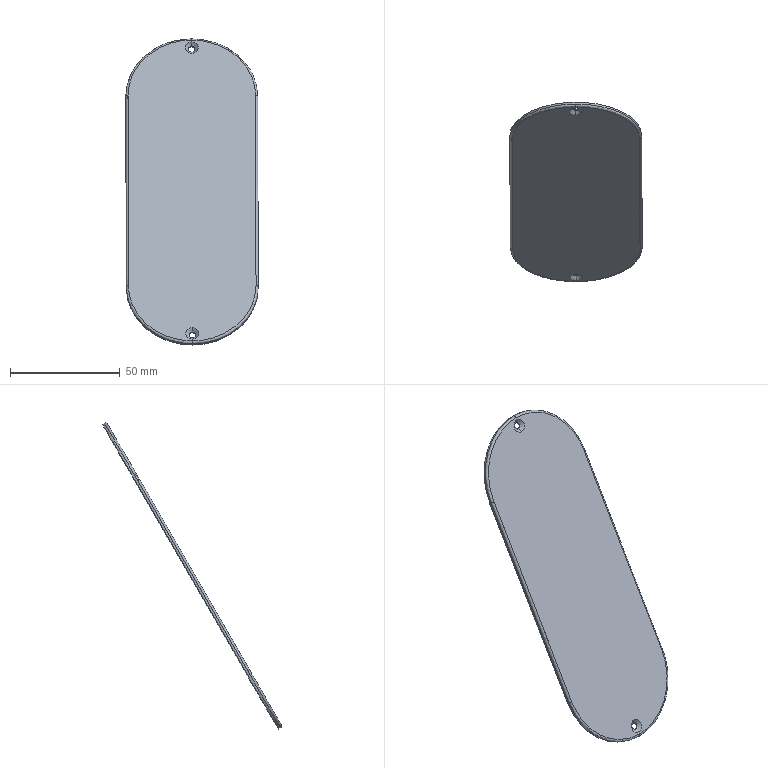Part | SolidWorks | features BaseBody 1 | 1 solid | 22 faces | box 60.221 x 81.366 x 139.198 mm | volume 17515 mm3 | cylinder 10 | spline 4 | cone 4 | plane 4 | commonest cylinder face diameters 3 x4 2 x3 60 x3
STEP:
#1=CARTESIAN_POINT('',(743.209,-1.322,-30.446));
#2=VERTEX_POINT('',#1);
#3=CARTESIAN_POINT('',(743.144,-1.322,-30.446));
#4=VERTEX_POINT('',#3);
#5=CARTESIAN_POINT('',(743.144,13.678,-4.465));
#6=DIRECTION('',(-0.003769,0.866,-0.5));
#7=DIRECTION('',(0.,-0.5,-0.866));
#8=AXIS2_PLACEMENT_3D('',#5,#6,#7);
#9=CIRCLE('',#8,30.);
#10=EDGE_CURVE('',#2,#4,#9,.T.);
#11=ORIENTED_EDGE('',*,*,#10,.F.);
#12=CARTESIAN_POINT('',(743.211,-1.688,-29.08));
#13=VERTEX_POINT('',#12);
#14=CARTESIAN_POINT('',(743.207,-0.8215,-29.58));
#15=DIRECTION('',(-1.,-0.004352,0.000000001));
#16=DIRECTION('',(0.002176,-0.5,-0.866));
#17=AXIS2_PLACEMENT_3D('',#14,#15,#16);
#18=CIRCLE('',#17,1.);
#19=EDGE_CURVE('',#2,#13,#18,.T.);
#20=ORIENTED_EDGE('',*,*,#19,.T.);
#21=CARTESIAN_POINT('',(714.148,12.686,-3.965));
#22=VERTEX_POINT('',#21);
#23=CARTESIAN_POINT('',(743.211,-1.688,-29.08));
#24=CARTESIAN_POINT('',(726.223,-1.761,-29.08));
#25=CARTESIAN_POINT('',(714.185,4.192,-18.677));
#26=CARTESIAN_POINT('',(714.148,12.686,-3.965));
#27=(BOUNDED_CURVE()B_SPLINE_CURVE(3,(#23,#24,#25,#26),.UNSPECIFIED.,.F.,.F.)B_SPLINE_CURVE_WITH_KNOTS((4,4),(0.,1.),.UNSPECIFIED.)CURVE()GEOMETRIC_REPRESENTATION_ITEM()RATIONAL_B_SPLINE_CURVE((1.,0.8047,0.8047,1.))REPRESENTATION_ITEM(''));
#28=EDGE_CURVE('',#13,#22,#27,.T.);
#29=ORIENTED_EDGE('',*,*,#28,.T.);
#30=CARTESIAN_POINT('',(714.144,12.686,-3.965));
#31=VERTEX_POINT('',#30);
#32=CARTESIAN_POINT('',(714.144,13.552,-4.465));
#33=DIRECTION('',(0.002176,-0.5,-0.866));
#34=DIRECTION('',(-1.,-0.004352,0.000000001));
#35=AXIS2_PLACEMENT_3D('',#32,#33,#34);
#36=CIRCLE('',#35,1.);
#37=EDGE_CURVE('',#22,#31,#36,.T.);
#38=ORIENTED_EDGE('',*,*,#37,.T.);
#39=CARTESIAN_POINT('',(713.144,13.548,-4.465));
#40=VERTEX_POINT('',#39);
#41=CARTESIAN_POINT('',(714.144,13.552,-4.465));
#42=DIRECTION('',(0.002176,-0.5,-0.866));
#43=DIRECTION('',(-1.,-0.004352,0.000000001));
#44=AXIS2_PLACEMENT_3D('',#41,#42,#43);
#45=CIRCLE('',#44,1.);
#46=EDGE_CURVE('',#31,#40,#45,.T.);
#47=ORIENTED_EDGE('',*,*,#46,.T.);
#48=CARTESIAN_POINT('',(743.144,13.678,-4.465));
#49=DIRECTION('',(-0.003769,0.866,-0.5));
#50=DIRECTION('',(0.,-0.5,-0.866));
#51=AXIS2_PLACEMENT_3D('',#48,#49,#50);
#52=CIRCLE('',#51,30.);
#53=EDGE_CURVE('',#4,#40,#52,.T.);
#54=ORIENTED_EDGE('',*,*,#53,.F.);
#55=EDGE_LOOP('',(#11,#20,#29,#38,#47,#54));
#56=FACE_OUTER_BOUND('',#55,.T.);
#57=CARTESIAN_POINT('',(743.209,-1.322,-30.446));
#58=CARTESIAN_POINT('',(725.636,-1.398,-30.446));
#59=CARTESIAN_POINT('',(713.182,4.761,-19.684));
#60=CARTESIAN_POINT('',(713.144,13.548,-4.465));
#61=CARTESIAN_POINT('',(743.211,-1.829,-30.153));
#62=CARTESIAN_POINT('',(725.638,-1.905,-30.153));
#63=CARTESIAN_POINT('',(713.185,4.254,-19.391));
#64=CARTESIAN_POINT('',(713.146,13.04,-4.172));
#65=CARTESIAN_POINT('',(743.212,-1.98,-29.587));
#66=CARTESIAN_POINT('',(725.881,-2.056,-29.587));
#67=CARTESIAN_POINT('',(713.6,4.018,-18.974));
#68=CARTESIAN_POINT('',(713.562,12.684,-3.965));
#69=CARTESIAN_POINT('',(743.211,-1.688,-29.08));
#70=CARTESIAN_POINT('',(726.223,-1.761,-29.08));
#71=CARTESIAN_POINT('',(714.185,4.192,-18.677));
#72=CARTESIAN_POINT('',(714.148,12.686,-3.965));
#73=(BOUNDED_SURFACE()B_SPLINE_SURFACE(3,3,((#57,#58,#59,#60),(#61,#62,#63,#64),(#65,#66,#67,#68),(#69,#70,#71,#72)),.UNSPECIFIED.,.F.,.F.,.T.)B_SPLINE_SURFACE_WITH_KNOTS((4,4),(4,4),(0.,1.),(0.,1.),.UNSPECIFIED.)GEOMETRIC_REPRESENTATION_ITEM()RATIONAL_B_SPLINE_SURFACE(((1.,0.8047,0.8047,1.),(0.8047,0.6476,0.6476,0.8047),(0.8047,0.6476,0.6476,0.8047),(1.,0.8047,0.8047,1.)))REPRESENTATION_ITEM('')SURFACE());
#74=ADVANCED_FACE('',(#56),#73,.T.);
#75=CARTESIAN_POINT('',(742.861,78.678,108.118));
#76=VERTEX_POINT('',#75);
#77=CARTESIAN_POINT('',(772.926,63.808,82.137));
#78=VERTEX_POINT('',#77);
#79=CARTESIAN_POINT('',(742.926,63.678,82.137));
#80=DIRECTION('',(-0.003769,0.866,-0.5));
#81=DIRECTION('',(0.,-0.5,-0.866));
#82=AXIS2_PLACEMENT_3D('',#79,#80,#81);
#83=CIRCLE('',#82,30.);
#84=EDGE_CURVE('',#76,#78,#83,.T.);
#85=ORIENTED_EDGE('',*,*,#84,.F.);
#86=CARTESIAN_POINT('',(742.867,77.312,107.752));
#87=VERTEX_POINT('',#86);
#88=CARTESIAN_POINT('',(742.863,78.178,107.252));
#89=DIRECTION('',(1.,0.004352,-0.000000001));
#90=DIRECTION('',(-0.002176,0.5,0.866));
#91=AXIS2_PLACEMENT_3D('',#88,#89,#90);
#92=CIRCLE('',#91,1.);
#93=EDGE_CURVE('',#76,#87,#92,.T.);
#94=ORIENTED_EDGE('',*,*,#93,.T.);
#95=CARTESIAN_POINT('',(771.93,62.938,82.637));
#96=VERTEX_POINT('',#95);
#97=CARTESIAN_POINT('',(742.867,77.312,107.752));
#98=CARTESIAN_POINT('',(759.855,77.386,107.752));
#99=CARTESIAN_POINT('',(771.893,71.432,97.349));
#100=CARTESIAN_POINT('',(771.93,62.938,82.637));
#101=(BOUNDED_CURVE()B_SPLINE_CURVE(3,(#97,#98,#99,#100),.UNSPECIFIED.,.F.,.F.)B_SPLINE_CURVE_WITH_KNOTS((4,4),(0.,1.),.UNSPECIFIED.)CURVE()GEOMETRIC_REPRESENTATION_ITEM()RATIONAL_B_SPLINE_CURVE((1.,0.8047,0.8047,1.))REPRESENTATION_ITEM(''));
#102=EDGE_CURVE('',#87,#96,#101,.T.);
#103=ORIENTED_EDGE('',*,*,#102,.T.);
#104=CARTESIAN_POINT('',(771.926,63.804,82.137));
#105=DIRECTION('',(0.002176,-0.5,-0.866));
#106=DIRECTION('',(0.,0.866,-0.5));
#107=AXIS2_PLACEMENT_3D('',#104,#105,#106);
#108=CIRCLE('',#107,1.);
#109=EDGE_CURVE('',#78,#96,#108,.T.);
#110=ORIENTED_EDGE('',*,*,#109,.F.);
#111=EDGE_LOOP('',(#85,#94,#103,#110));
#112=FACE_OUTER_BOUND('',#111,.T.);
#113=CARTESIAN_POINT('',(742.861,78.678,108.118));
#114=CARTESIAN_POINT('',(760.434,78.754,108.118));
#115=CARTESIAN_POINT('',(772.888,72.595,97.357));
#116=CARTESIAN_POINT('',(772.926,63.808,82.137));
#117=CARTESIAN_POINT('',(742.863,78.17,108.411));
#118=CARTESIAN_POINT('',(760.437,78.247,108.411));
#119=CARTESIAN_POINT('',(772.89,72.088,97.649));
#120=CARTESIAN_POINT('',(772.928,63.301,82.43));
#121=CARTESIAN_POINT('',(742.866,77.605,108.259));
#122=CARTESIAN_POINT('',(760.197,77.68,108.259));
#123=CARTESIAN_POINT('',(772.478,71.606,97.646));
#124=CARTESIAN_POINT('',(772.516,62.941,82.637));
#125=CARTESIAN_POINT('',(742.867,77.312,107.752));
#126=CARTESIAN_POINT('',(759.855,77.386,107.752));
#127=CARTESIAN_POINT('',(771.893,71.432,97.349));
#128=CARTESIAN_POINT('',(771.93,62.938,82.637));
#129=(BOUNDED_SURFACE()B_SPLINE_SURFACE(3,3,((#113,#114,#115,#116),(#117,#118,#119,#120),(#121,#122,#123,#124),(#125,#126,#127,#128)),.UNSPECIFIED.,.F.,.F.,.F.)B_SPLINE_SURFACE_WITH_KNOTS((4,4),(4,4),(0.,1.),(0.,1.),.UNSPECIFIED.)GEOMETRIC_REPRESENTATION_ITEM()RATIONAL_B_SPLINE_SURFACE(((1.,0.8047,0.8047,1.),(0.8047,0.6476,0.6476,0.8047),(0.8047,0.6476,0.6476,0.8047),(1.,0.8047,0.8047,1.)))REPRESENTATION_ITEM('')SURFACE());
#130=ADVANCED_FACE('',(#112),#129,.T.);
#131=CARTESIAN_POINT('',(713.14,14.414,-4.965));
#132=VERTEX_POINT('',#131);
#133=CARTESIAN_POINT('',(743.14,-0.4558,-30.946));
#134=VERTEX_POINT('',#133);
#135=CARTESIAN_POINT('',(743.14,14.544,-4.965));
#136=DIRECTION('',(0.003769,-0.866,0.5));
#137=DIRECTION('',(0.,-0.5,-0.866));
#138=AXIS2_PLACEMENT_3D('',#135,#136,#137);
#139=CIRCLE('',#138,30.);
#140=EDGE_CURVE('',#132,#134,#139,.T.);
#141=ORIENTED_EDGE('',*,*,#140,.T.);
#142=CARTESIAN_POINT('',(743.14,-0.4558,-30.946));
#143=DIRECTION('',(0.003769,-0.866,0.5));
#144=VECTOR('',#143,1000.);
#145=LINE('',#142,#144);
#146=EDGE_CURVE('',#134,#4,#145,.T.);
#147=ORIENTED_EDGE('',*,*,#146,.T.);
#148=ORIENTED_EDGE('',*,*,#53,.T.);
#149=CARTESIAN_POINT('',(713.14,14.414,-4.965));
#150=DIRECTION('',(-0.003769,0.866,-0.5));
#151=VECTOR('',#150,1000.);
#152=LINE('',#149,#151);
#153=EDGE_CURVE('',#40,#132,#152,.T.);
#154=ORIENTED_EDGE('',*,*,#153,.T.);
#155=EDGE_LOOP('',(#141,#147,#148,#154));
#156=FACE_OUTER_BOUND('',#155,.T.);
#157=CARTESIAN_POINT('',(743.14,14.544,-4.965));
#158=DIRECTION('',(0.003769,-0.866,0.5));
#159=DIRECTION('',(0.,-0.5,-0.866));
#160=AXIS2_PLACEMENT_3D('',#157,#158,#159);
#161=CYLINDRICAL_SURFACE('',#160,30.);
#162=ADVANCED_FACE('',(#156),#161,.T.);
#163=CARTESIAN_POINT('',(742.87,75.861,102.239));
#164=VERTEX_POINT('',#163);
#165=CARTESIAN_POINT('',(742.87,77.361,104.837));
#166=VERTEX_POINT('',#165);
#167=CARTESIAN_POINT('',(742.87,76.611,103.538));
#168=DIRECTION('',(-0.003769,0.866,-0.5));
#169=DIRECTION('',(0.,0.5,0.866));
#170=AXIS2_PLACEMENT_3D('',#167,#168,#169);
#171=CIRCLE('',#170,1.5);
#172=EDGE_CURVE('',#164,#166,#171,.T.);
#173=ORIENTED_EDGE('',*,*,#172,.F.);
#174=CARTESIAN_POINT('',(742.868,76.294,101.989));
#175=VERTEX_POINT('',#174);
#176=CARTESIAN_POINT('',(742.868,76.294,101.989));
#177=DIRECTION('',(-0.003769,0.866,-0.5));
#178=VECTOR('',#177,1000.);
#179=LINE('',#176,#178);
#180=EDGE_CURVE('',#164,#175,#179,.T.);
#181=ORIENTED_EDGE('',*,*,#180,.T.);
#182=CARTESIAN_POINT('',(742.868,77.794,104.587));
#183=VERTEX_POINT('',#182);
#184=CARTESIAN_POINT('',(742.868,77.044,103.288));
#185=DIRECTION('',(-0.003769,0.866,-0.5));
#186=DIRECTION('',(0.,0.5,0.866));
#187=AXIS2_PLACEMENT_3D('',#184,#185,#186);
#188=CIRCLE('',#187,1.5);
#189=EDGE_CURVE('',#175,#183,#188,.T.);
#190=ORIENTED_EDGE('',*,*,#189,.T.);
#191=CARTESIAN_POINT('',(742.868,77.794,104.587));
#192=DIRECTION('',(-0.003769,0.866,-0.5));
#193=VECTOR('',#192,1000.);
#194=LINE('',#191,#193);
#195=EDGE_CURVE('',#166,#183,#194,.T.);
#196=ORIENTED_EDGE('',*,*,#195,.F.);
#197=EDGE_LOOP('',(#173,#181,#190,#196));
#198=FACE_OUTER_BOUND('',#197,.T.);
#199=CARTESIAN_POINT('',(742.868,77.044,103.288));
#200=DIRECTION('',(-0.003769,0.866,-0.5));
#201=DIRECTION('',(0.,0.5,0.866));
#202=AXIS2_PLACEMENT_3D('',#199,#200,#201);
#203=CYLINDRICAL_SURFACE('',#202,1.5);
#204=ADVANCED_FACE('',(#198),#203,.F.);
#205=CARTESIAN_POINT('',(743.196,0.8614,-27.665));
#206=VERTEX_POINT('',#205);
#207=CARTESIAN_POINT('',(743.196,2.361,-25.067));
#208=VERTEX_POINT('',#207);
#209=CARTESIAN_POINT('',(743.196,1.611,-26.366));
#210=DIRECTION('',(-0.003769,0.866,-0.5));
#211=DIRECTION('',(0.,0.5,0.866));
#212=AXIS2_PLACEMENT_3D('',#209,#210,#211);
#213=CIRCLE('',#212,1.5);
#214=EDGE_CURVE('',#206,#208,#213,.T.);
#215=ORIENTED_EDGE('',*,*,#214,.F.);
#216=CARTESIAN_POINT('',(743.195,1.294,-27.915));
#217=VERTEX_POINT('',#216);
#218=CARTESIAN_POINT('',(743.195,1.294,-27.915));
#219=DIRECTION('',(-0.003769,0.866,-0.5));
#220=VECTOR('',#219,1000.);
#221=LINE('',#218,#220);
#222=EDGE_CURVE('',#206,#217,#221,.T.);
#223=ORIENTED_EDGE('',*,*,#222,.T.);
#224=CARTESIAN_POINT('',(743.195,2.794,-25.317));
#225=VERTEX_POINT('',#224);
#226=CARTESIAN_POINT('',(743.195,2.044,-26.616));
#227=DIRECTION('',(-0.003769,0.866,-0.5));
#228=DIRECTION('',(0.,0.5,0.866));
#229=AXIS2_PLACEMENT_3D('',#226,#227,#228);
#230=CIRCLE('',#229,1.5);
#231=EDGE_CURVE('',#217,#225,#230,.T.);
#232=ORIENTED_EDGE('',*,*,#231,.T.);
#233=CARTESIAN_POINT('',(743.195,2.794,-25.317));
#234=DIRECTION('',(-0.003769,0.866,-0.5));
#235=VECTOR('',#234,1000.);
#236=LINE('',#233,#235);
#237=EDGE_CURVE('',#208,#225,#236,.T.);
#238=ORIENTED_EDGE('',*,*,#237,.F.);
#239=EDGE_LOOP('',(#215,#223,#232,#238));
#240=FACE_OUTER_BOUND('',#239,.T.);
#241=CARTESIAN_POINT('',(743.195,2.044,-26.616));
#242=DIRECTION('',(-0.003769,0.866,-0.5));
#243=DIRECTION('',(0.,0.5,0.866));
#244=AXIS2_PLACEMENT_3D('',#241,#242,#243);
#245=CYLINDRICAL_SURFACE('',#244,1.5);
#246=ADVANCED_FACE('',(#240),#245,.F.);
#247=ORIENTED_EDGE('',*,*,#46,.F.);
#248=CARTESIAN_POINT('',(713.927,62.686,82.637));
#249=VERTEX_POINT('',#248);
#250=CARTESIAN_POINT('',(714.09,25.186,17.685));
#251=DIRECTION('',(-0.002176,0.5,0.866));
#252=VECTOR('',#251,1000.);
#253=LINE('',#250,#252);
#254=EDGE_CURVE('',#31,#249,#253,.T.);
#255=ORIENTED_EDGE('',*,*,#254,.T.);
#256=CARTESIAN_POINT('',(712.927,63.547,82.137));
#257=VERTEX_POINT('',#256);
#258=CARTESIAN_POINT('',(713.927,63.552,82.137));
#259=DIRECTION('',(0.002176,-0.5,-0.866));
#260=DIRECTION('',(0.,-0.866,0.5));
#261=AXIS2_PLACEMENT_3D('',#258,#259,#260);
#262=CIRCLE('',#261,1.);
#263=EDGE_CURVE('',#249,#257,#262,.T.);
#264=ORIENTED_EDGE('',*,*,#263,.T.);
#265=CARTESIAN_POINT('',(713.144,13.548,-4.465));
#266=DIRECTION('',(-0.002176,0.5,0.866));
#267=VECTOR('',#266,1000.);
#268=LINE('',#265,#267);
#269=EDGE_CURVE('',#40,#257,#268,.T.);
#270=ORIENTED_EDGE('',*,*,#269,.F.);
#271=EDGE_LOOP('',(#247,#255,#264,#270));
#272=FACE_OUTER_BOUND('',#271,.T.);
#273=CARTESIAN_POINT('',(714.09,26.052,17.185));
#274=DIRECTION('',(-0.002176,0.5,0.866));
#275=DIRECTION('',(0.,-0.866,0.5));
#276=AXIS2_PLACEMENT_3D('',#273,#274,#275);
#277=CYLINDRICAL_SURFACE('',#276,1.);
#278=ADVANCED_FACE('',(#272),#277,.T.);
#279=ORIENTED_EDGE('',*,*,#172,.T.);
#280=CARTESIAN_POINT('',(742.876,76.812,106.886));
#281=VERTEX_POINT('',#280);
#282=CARTESIAN_POINT('',(742.876,76.812,106.886));
#283=DIRECTION('',(0.002665,-0.2588,0.9659));
#284=VECTOR('',#283,1000.);
#285=LINE('',#282,#284);
#286=EDGE_CURVE('',#166,#281,#285,.T.);
#287=ORIENTED_EDGE('',*,*,#286,.T.);
#288=CARTESIAN_POINT('',(742.876,73.812,101.69));
#289=VERTEX_POINT('',#288);
#290=CARTESIAN_POINT('',(742.876,75.312,104.288));
#291=DIRECTION('',(-0.003769,0.866,-0.5));
#292=DIRECTION('',(0.,-0.5,-0.866));
#293=AXIS2_PLACEMENT_3D('',#290,#291,#292);
#294=CIRCLE('',#293,3.);
#295=EDGE_CURVE('',#289,#281,#294,.T.);
#296=ORIENTED_EDGE('',*,*,#295,.F.);
#297=CARTESIAN_POINT('',(742.876,73.812,101.69));
#298=DIRECTION('',(0.002665,-0.9659,-0.2588));
#299=VECTOR('',#298,1000.);
#300=LINE('',#297,#299);
#301=EDGE_CURVE('',#164,#289,#300,.T.);
#302=ORIENTED_EDGE('',*,*,#301,.F.);
#303=EDGE_LOOP('',(#279,#287,#296,#302));
#304=FACE_OUTER_BOUND('',#303,.T.);
#305=CARTESIAN_POINT('',(742.876,75.312,104.288));
#306=DIRECTION('',(0.003769,-0.866,0.5));
#307=DIRECTION('',(0.,-0.5,-0.866));
#308=AXIS2_PLACEMENT_3D('',#305,#306,#307);
#309=CONICAL_SURFACE('',#308,3.,0.7854);
#310=ADVANCED_FACE('',(#304),#309,.F.);
#311=ORIENTED_EDGE('',*,*,#214,.T.);
#312=CARTESIAN_POINT('',(743.202,1.812,-23.018));
#313=VERTEX_POINT('',#312);
#314=CARTESIAN_POINT('',(743.202,1.812,-23.018));
#315=DIRECTION('',(0.002665,-0.2588,0.9659));
#316=VECTOR('',#315,1000.);
#317=LINE('',#314,#316);
#318=EDGE_CURVE('',#208,#313,#317,.T.);
#319=ORIENTED_EDGE('',*,*,#318,.T.);
#320=CARTESIAN_POINT('',(743.202,-1.188,-28.214));
#321=VERTEX_POINT('',#320);
#322=CARTESIAN_POINT('',(743.202,0.3124,-25.616));
#323=DIRECTION('',(-0.003769,0.866,-0.5));
#324=DIRECTION('',(0.,-0.5,-0.866));
#325=AXIS2_PLACEMENT_3D('',#322,#323,#324);
#326=CIRCLE('',#325,3.);
#327=EDGE_CURVE('',#321,#313,#326,.T.);
#328=ORIENTED_EDGE('',*,*,#327,.F.);
#329=CARTESIAN_POINT('',(743.202,-1.188,-28.214));
#330=DIRECTION('',(0.002665,-0.9659,-0.2588));
#331=VECTOR('',#330,1000.);
#332=LINE('',#329,#331);
#333=EDGE_CURVE('',#206,#321,#332,.T.);
#334=ORIENTED_EDGE('',*,*,#333,.F.);
#335=EDGE_LOOP('',(#311,#319,#328,#334));
#336=FACE_OUTER_BOUND('',#335,.T.);
#337=CARTESIAN_POINT('',(743.202,0.3124,-25.616));
#338=DIRECTION('',(0.003769,-0.866,0.5));
#339=DIRECTION('',(0.,-0.5,-0.866));
#340=AXIS2_PLACEMENT_3D('',#337,#338,#339);
#341=CONICAL_SURFACE('',#340,3.,0.7854);
#342=ADVANCED_FACE('',(#336),#341,.F.);
#343=CARTESIAN_POINT('',(773.14,14.675,-4.965));
#344=VERTEX_POINT('',#343);
#345=CARTESIAN_POINT('',(772.922,64.674,81.637));
#346=VERTEX_POINT('',#345);
#347=CARTESIAN_POINT('',(773.14,14.675,-4.965));
#348=DIRECTION('',(-0.002176,0.5,0.866));
#349=VECTOR('',#348,1000.);
#350=LINE('',#347,#349);
#351=EDGE_CURVE('',#344,#346,#350,.T.);
#352=ORIENTED_EDGE('',*,*,#351,.F.);
#353=CARTESIAN_POINT('',(743.14,14.544,-4.965));
#354=DIRECTION('',(0.003769,-0.866,0.5));
#355=DIRECTION('',(0.,-0.5,-0.866));
#356=AXIS2_PLACEMENT_3D('',#353,#354,#355);
#357=CIRCLE('',#356,30.);
#358=EDGE_CURVE('',#134,#344,#357,.T.);
#359=ORIENTED_EDGE('',*,*,#358,.F.);
#360=ORIENTED_EDGE('',*,*,#140,.F.);
#361=CARTESIAN_POINT('',(712.923,64.413,81.637));
#362=VERTEX_POINT('',#361);
#363=CARTESIAN_POINT('',(712.923,64.413,81.637));
#364=DIRECTION('',(0.002176,-0.5,-0.866));
#365=VECTOR('',#364,1000.);
#366=LINE('',#363,#365);
#367=EDGE_CURVE('',#362,#132,#366,.T.);
#368=ORIENTED_EDGE('',*,*,#367,.F.);
#369=CARTESIAN_POINT('',(742.923,64.544,81.637));
#370=DIRECTION('',(0.003769,-0.866,0.5));
#371=DIRECTION('',(0.,-0.5,-0.866));
#372=AXIS2_PLACEMENT_3D('',#369,#370,#371);
#373=CIRCLE('',#372,30.);
#374=EDGE_CURVE('',#346,#362,#373,.T.);
#375=ORIENTED_EDGE('',*,*,#374,.F.);
#376=EDGE_LOOP('',(#352,#359,#360,#368,#375));
#377=FACE_OUTER_BOUND('',#376,.T.);
#378=CARTESIAN_POINT('',(742.868,77.044,103.288));
#379=DIRECTION('',(-0.003769,0.866,-0.5));
#380=DIRECTION('',(0.,0.5,0.866));
#381=AXIS2_PLACEMENT_3D('',#378,#379,#380);
#382=CIRCLE('',#381,1.5);
#383=EDGE_CURVE('',#183,#175,#382,.T.);
#384=ORIENTED_EDGE('',*,*,#383,.F.);
#385=ORIENTED_EDGE('',*,*,#189,.F.);
#386=EDGE_LOOP('',(#384,#385));
#387=FACE_BOUND('',#386,.T.);
#388=CARTESIAN_POINT('',(743.195,2.044,-26.616));
#389=DIRECTION('',(-0.003769,0.866,-0.5));
#390=DIRECTION('',(0.,0.5,0.866));
#391=AXIS2_PLACEMENT_3D('',#388,#389,#390);
#392=CIRCLE('',#391,1.5);
#393=EDGE_CURVE('',#225,#217,#392,.T.);
#394=ORIENTED_EDGE('',*,*,#393,.F.);
#395=ORIENTED_EDGE('',*,*,#231,.F.);
#396=EDGE_LOOP('',(#394,#395));
#397=FACE_BOUND('',#396,.T.);
#398=CARTESIAN_POINT('',(743.031,39.544,38.336));
#399=DIRECTION('',(0.003769,-0.866,0.5));
#400=DIRECTION('',(0.,-0.5,-0.866));
#401=AXIS2_PLACEMENT_3D('',#398,#399,#400);
#402=PLANE('',#401);
#403=ADVANCED_FACE('',(#377,#387,#397),#402,.F.);
#404=ORIENTED_EDGE('',*,*,#351,.T.);
#405=CARTESIAN_POINT('',(772.922,64.674,81.637));
#406=DIRECTION('',(0.003769,-0.866,0.5));
#407=VECTOR('',#406,1000.);
#408=LINE('',#405,#407);
#409=EDGE_CURVE('',#346,#78,#408,.T.);
#410=ORIENTED_EDGE('',*,*,#409,.T.);
#411=CARTESIAN_POINT('',(773.144,13.809,-4.465));
#412=VERTEX_POINT('',#411);
#413=CARTESIAN_POINT('',(772.926,63.808,82.137));
#414=DIRECTION('',(0.002176,-0.5,-0.866));
#415=VECTOR('',#414,1000.);
#416=LINE('',#413,#415);
#417=EDGE_CURVE('',#78,#412,#416,.T.);
#418=ORIENTED_EDGE('',*,*,#417,.T.);
#419=CARTESIAN_POINT('',(773.144,13.809,-4.465));
#420=DIRECTION('',(-0.003769,0.866,-0.5));
#421=VECTOR('',#420,1000.);
#422=LINE('',#419,#421);
#423=EDGE_CURVE('',#412,#344,#422,.T.);
#424=ORIENTED_EDGE('',*,*,#423,.T.);
#425=EDGE_LOOP('',(#404,#410,#418,#424));
#426=FACE_OUTER_BOUND('',#425,.T.);
#427=CARTESIAN_POINT('',(772.922,64.674,81.637));
#428=DIRECTION('',(1.,0.004352,-0.000000001));
#429=DIRECTION('',(-0.004352,1.,0.));
#430=AXIS2_PLACEMENT_3D('',#427,#428,#429);
#431=PLANE('',#430);
#432=ADVANCED_FACE('',(#426),#431,.T.);
#433=ORIENTED_EDGE('',*,*,#146,.F.);
#434=ORIENTED_EDGE('',*,*,#358,.T.);
#435=ORIENTED_EDGE('',*,*,#423,.F.);
#436=CARTESIAN_POINT('',(743.144,13.678,-4.465));
#437=DIRECTION('',(-0.003769,0.866,-0.5));
#438=DIRECTION('',(0.,-0.5,-0.866));
#439=AXIS2_PLACEMENT_3D('',#436,#437,#438);
#440=CIRCLE('',#439,30.);
#441=EDGE_CURVE('',#412,#2,#440,.T.);
#442=ORIENTED_EDGE('',*,*,#441,.T.);
#443=ORIENTED_EDGE('',*,*,#10,.T.);
#444=EDGE_LOOP('',(#433,#434,#435,#442,#443));
#445=FACE_OUTER_BOUND('',#444,.T.);
#446=CARTESIAN_POINT('',(743.14,14.544,-4.965));
#447=DIRECTION('',(0.003769,-0.866,0.5));
#448=DIRECTION('',(0.,-0.5,-0.866));
#449=AXIS2_PLACEMENT_3D('',#446,#447,#448);
#450=CYLINDRICAL_SURFACE('',#449,30.);
#451=ADVANCED_FACE('',(#445),#450,.T.);
#452=ORIENTED_EDGE('',*,*,#367,.T.);
#453=ORIENTED_EDGE('',*,*,#153,.F.);
#454=ORIENTED_EDGE('',*,*,#269,.T.);
#455=CARTESIAN_POINT('',(712.927,63.547,82.137));
#456=DIRECTION('',(-0.003769,0.866,-0.5));
#457=VECTOR('',#456,1000.);
#458=LINE('',#455,#457);
#459=EDGE_CURVE('',#257,#362,#458,.T.);
#460=ORIENTED_EDGE('',*,*,#459,.T.);
#461=EDGE_LOOP('',(#452,#453,#454,#460));
#462=FACE_OUTER_BOUND('',#461,.T.);
#463=CARTESIAN_POINT('',(713.14,14.414,-4.965));
#464=DIRECTION('',(-1.,-0.004352,0.000000001));
#465=DIRECTION('',(0.004352,-1.,0.));
#466=AXIS2_PLACEMENT_3D('',#463,#464,#465);
#467=PLANE('',#466);
#468=ADVANCED_FACE('',(#462),#467,.T.);
#469=ORIENTED_EDGE('',*,*,#459,.F.);
#470=CARTESIAN_POINT('',(742.926,63.678,82.137));
#471=DIRECTION('',(-0.003769,0.866,-0.5));
#472=DIRECTION('',(0.,-0.5,-0.866));
#473=AXIS2_PLACEMENT_3D('',#470,#471,#472);
#474=CIRCLE('',#473,30.);
#475=EDGE_CURVE('',#257,#76,#474,.T.);
#476=ORIENTED_EDGE('',*,*,#475,.T.);
#477=ORIENTED_EDGE('',*,*,#84,.T.);
#478=ORIENTED_EDGE('',*,*,#409,.F.);
#479=ORIENTED_EDGE('',*,*,#374,.T.);
#480=EDGE_LOOP('',(#469,#476,#477,#478,#479));
#481=FACE_OUTER_BOUND('',#480,.T.);
#482=CARTESIAN_POINT('',(742.923,64.544,81.637));
#483=DIRECTION('',(0.003769,-0.866,0.5));
#484=DIRECTION('',(0.,-0.5,-0.866));
#485=AXIS2_PLACEMENT_3D('',#482,#483,#484);
#486=CYLINDRICAL_SURFACE('',#485,30.);
#487=ADVANCED_FACE('',(#481),#486,.T.);
#488=ORIENTED_EDGE('',*,*,#180,.F.);
#489=CARTESIAN_POINT('',(742.87,76.611,103.538));
#490=DIRECTION('',(-0.003769,0.866,-0.5));
#491=DIRECTION('',(0.,0.5,0.866));
#492=AXIS2_PLACEMENT_3D('',#489,#490,#491);
#493=CIRCLE('',#492,1.5);
#494=EDGE_CURVE('',#166,#164,#493,.T.);
#495=ORIENTED_EDGE('',*,*,#494,.F.);
#496=ORIENTED_EDGE('',*,*,#195,.T.);
#497=ORIENTED_EDGE('',*,*,#383,.T.);
#498=EDGE_LOOP('',(#488,#495,#496,#497));
#499=FACE_OUTER_BOUND('',#498,.T.);
#500=CARTESIAN_POINT('',(742.868,77.044,103.288));
#501=DIRECTION('',(-0.003769,0.866,-0.5));
#502=DIRECTION('',(0.,0.5,0.866));
#503=AXIS2_PLACEMENT_3D('',#500,#501,#502);
#504=CYLINDRICAL_SURFACE('',#503,1.5);
#505=ADVANCED_FACE('',(#499),#504,.F.);
#506=ORIENTED_EDGE('',*,*,#222,.F.);
#507=CARTESIAN_POINT('',(743.196,1.611,-26.366));
#508=DIRECTION('',(-0.003769,0.866,-0.5));
#509=DIRECTION('',(0.,0.5,0.866));
#510=AXIS2_PLACEMENT_3D('',#507,#508,#509);
#511=CIRCLE('',#510,1.5);
#512=EDGE_CURVE('',#208,#206,#511,.T.);
#513=ORIENTED_EDGE('',*,*,#512,.F.);
#514=ORIENTED_EDGE('',*,*,#237,.T.);
#515=ORIENTED_EDGE('',*,*,#393,.T.);
#516=EDGE_LOOP('',(#506,#513,#514,#515));
#517=FACE_OUTER_BOUND('',#516,.T.);
#518=CARTESIAN_POINT('',(743.195,2.044,-26.616));
#519=DIRECTION('',(-0.003769,0.866,-0.5));
#520=DIRECTION('',(0.,0.5,0.866));
#521=AXIS2_PLACEMENT_3D('',#518,#519,#520);
#522=CYLINDRICAL_SURFACE('',#521,1.5);
#523=ADVANCED_FACE('',(#517),#522,.F.);
#524=ORIENTED_EDGE('',*,*,#417,.F.);
#525=ORIENTED_EDGE('',*,*,#109,.T.);
#526=CARTESIAN_POINT('',(772.147,12.939,-3.965));
#527=VERTEX_POINT('',#526);
#528=CARTESIAN_POINT('',(771.984,50.438,60.987));
#529=DIRECTION('',(0.002176,-0.5,-0.866));
#530=VECTOR('',#529,1000.);
#531=LINE('',#528,#530);
#532=EDGE_CURVE('',#96,#527,#531,.T.);
#533=ORIENTED_EDGE('',*,*,#532,.T.);
#534=CARTESIAN_POINT('',(772.144,13.805,-4.465));
#535=DIRECTION('',(-0.002176,0.5,0.866));
#536=DIRECTION('',(0.,0.866,-0.5));
#537=AXIS2_PLACEMENT_3D('',#534,#535,#536);
#538=CIRCLE('',#537,1.);
#539=EDGE_CURVE('',#527,#412,#538,.T.);
#540=ORIENTED_EDGE('',*,*,#539,.T.);
#541=EDGE_LOOP('',(#524,#525,#533,#540));
#542=FACE_OUTER_BOUND('',#541,.T.);
#543=CARTESIAN_POINT('',(771.98,51.304,60.487));
#544=DIRECTION('',(0.002176,-0.5,-0.866));
#545=DIRECTION('',(0.,0.866,-0.5));
#546=AXIS2_PLACEMENT_3D('',#543,#544,#545);
#547=CYLINDRICAL_SURFACE('',#546,1.);
#548=ADVANCED_FACE('',(#542),#547,.T.);
#549=ORIENTED_EDGE('',*,*,#19,.F.);
#550=ORIENTED_EDGE('',*,*,#441,.F.);
#551=ORIENTED_EDGE('',*,*,#539,.F.);
#552=CARTESIAN_POINT('',(772.147,12.939,-3.965));
#553=CARTESIAN_POINT('',(772.184,4.445,-18.677));
#554=CARTESIAN_POINT('',(760.198,-1.614,-29.08));
#555=CARTESIAN_POINT('',(743.211,-1.688,-29.08));
#556=(BOUNDED_CURVE()B_SPLINE_CURVE(3,(#552,#553,#554,#555),.UNSPECIFIED.,.F.,.F.)B_SPLINE_CURVE_WITH_KNOTS((4,4),(0.,1.),.UNSPECIFIED.)CURVE()GEOMETRIC_REPRESENTATION_ITEM()RATIONAL_B_SPLINE_CURVE((1.,0.8047,0.8047,1.))REPRESENTATION_ITEM(''));
#557=EDGE_CURVE('',#527,#13,#556,.T.);
#558=ORIENTED_EDGE('',*,*,#557,.T.);
#559=EDGE_LOOP('',(#549,#550,#551,#558));
#560=FACE_OUTER_BOUND('',#559,.T.);
#561=CARTESIAN_POINT('',(773.144,13.809,-4.465));
#562=CARTESIAN_POINT('',(773.182,5.022,-19.684));
#563=CARTESIAN_POINT('',(760.783,-1.245,-30.446));
#564=CARTESIAN_POINT('',(743.209,-1.322,-30.446));
#565=CARTESIAN_POINT('',(773.146,13.302,-4.172));
#566=CARTESIAN_POINT('',(773.184,4.515,-19.391));
#567=CARTESIAN_POINT('',(760.785,-1.752,-30.153));
#568=CARTESIAN_POINT('',(743.211,-1.829,-30.153));
#569=CARTESIAN_POINT('',(772.733,12.941,-3.965));
#570=CARTESIAN_POINT('',(772.771,4.276,-18.974));
#571=CARTESIAN_POINT('',(760.543,-1.905,-29.587));
#572=CARTESIAN_POINT('',(743.212,-1.98,-29.587));
#573=CARTESIAN_POINT('',(772.147,12.939,-3.965));
#574=CARTESIAN_POINT('',(772.184,4.445,-18.677));
#575=CARTESIAN_POINT('',(760.198,-1.614,-29.08));
#576=CARTESIAN_POINT('',(743.211,-1.688,-29.08));
#577=(BOUNDED_SURFACE()B_SPLINE_SURFACE(3,3,((#561,#562,#563,#564),(#565,#566,#567,#568),(#569,#570,#571,#572),(#573,#574,#575,#576)),.UNSPECIFIED.,.F.,.F.,.T.)B_SPLINE_SURFACE_WITH_KNOTS((4,4),(4,4),(0.,1.),(0.,1.),.UNSPECIFIED.)GEOMETRIC_REPRESENTATION_ITEM()RATIONAL_B_SPLINE_SURFACE(((1.,0.8047,0.8047,1.),(0.8047,0.6476,0.6476,0.8047),(0.8047,0.6476,0.6476,0.8047),(1.,0.8047,0.8047,1.)))REPRESENTATION_ITEM('')SURFACE());
#578=ADVANCED_FACE('',(#560),#577,.T.);
#579=ORIENTED_EDGE('',*,*,#254,.F.);
#580=ORIENTED_EDGE('',*,*,#37,.F.);
#581=CARTESIAN_POINT('',(713.93,62.686,82.637));
#582=VERTEX_POINT('',#581);
#583=CARTESIAN_POINT('',(713.93,62.686,82.637));
#584=DIRECTION('',(0.002176,-0.5,-0.866));
#585=VECTOR('',#584,1000.);
#586=LINE('',#583,#585);
#587=EDGE_CURVE('',#582,#22,#586,.T.);
#588=ORIENTED_EDGE('',*,*,#587,.F.);
#589=CARTESIAN_POINT('',(713.927,63.552,82.137));
#590=DIRECTION('',(0.002176,-0.5,-0.866));
#591=DIRECTION('',(0.000000001,-0.866,0.5));
#592=AXIS2_PLACEMENT_3D('',#589,#590,#591);
#593=CIRCLE('',#592,1.);
#594=EDGE_CURVE('',#582,#249,#593,.T.);
#595=ORIENTED_EDGE('',*,*,#594,.T.);
#596=EDGE_LOOP('',(#579,#580,#588,#595));
#597=FACE_OUTER_BOUND('',#596,.T.);
#598=CARTESIAN_POINT('',(714.09,26.052,17.185));
#599=DIRECTION('',(-0.002176,0.5,0.866));
#600=DIRECTION('',(0.,-0.866,0.5));
#601=AXIS2_PLACEMENT_3D('',#598,#599,#600);
#602=CYLINDRICAL_SURFACE('',#601,1.);
#603=ADVANCED_FACE('',(#597),#602,.T.);
#604=ORIENTED_EDGE('',*,*,#93,.F.);
#605=ORIENTED_EDGE('',*,*,#475,.F.);
#606=ORIENTED_EDGE('',*,*,#263,.F.);
#607=ORIENTED_EDGE('',*,*,#594,.F.);
#608=CARTESIAN_POINT('',(713.93,62.686,82.637));
#609=CARTESIAN_POINT('',(713.893,71.179,97.349));
#610=CARTESIAN_POINT('',(725.879,77.238,107.752));
#611=CARTESIAN_POINT('',(742.867,77.312,107.752));
#612=(BOUNDED_CURVE()B_SPLINE_CURVE(3,(#608,#609,#610,#611),.UNSPECIFIED.,.F.,.T.)B_SPLINE_CURVE_WITH_KNOTS((4,4),(0.,1.),.UNSPECIFIED.)CURVE()GEOMETRIC_REPRESENTATION_ITEM()RATIONAL_B_SPLINE_CURVE((1.,0.8047,0.8047,1.))REPRESENTATION_ITEM(''));
#613=EDGE_CURVE('',#582,#87,#612,.T.);
#614=ORIENTED_EDGE('',*,*,#613,.T.);
#615=EDGE_LOOP('',(#604,#605,#606,#607,#614));
#616=FACE_OUTER_BOUND('',#615,.T.);
#617=CARTESIAN_POINT('',(712.927,63.547,82.137));
#618=CARTESIAN_POINT('',(712.888,72.334,97.357));
#619=CARTESIAN_POINT('',(725.288,78.601,108.118));
#620=CARTESIAN_POINT('',(742.861,78.678,108.118));
#621=CARTESIAN_POINT('',(712.929,63.04,82.43));
#622=CARTESIAN_POINT('',(712.891,71.827,97.649));
#623=CARTESIAN_POINT('',(725.29,78.094,108.411));
#624=CARTESIAN_POINT('',(742.863,78.17,108.411));
#625=CARTESIAN_POINT('',(713.345,62.683,82.637));
#626=CARTESIAN_POINT('',(713.307,71.348,97.646));
#627=CARTESIAN_POINT('',(725.535,77.529,108.259));
#628=CARTESIAN_POINT('',(742.866,77.605,108.259));
#629=CARTESIAN_POINT('',(713.93,62.686,82.637));
#630=CARTESIAN_POINT('',(713.893,71.179,97.349));
#631=CARTESIAN_POINT('',(725.879,77.238,107.752));
#632=CARTESIAN_POINT('',(742.867,77.312,107.752));
#633=(BOUNDED_SURFACE()B_SPLINE_SURFACE(3,3,((#617,#618,#619,#620),(#621,#622,#623,#624),(#625,#626,#627,#628),(#629,#630,#631,#632)),.UNSPECIFIED.,.F.,.F.,.T.)B_SPLINE_SURFACE_WITH_KNOTS((4,4),(4,4),(0.,1.),(0.,1.),.UNSPECIFIED.)GEOMETRIC_REPRESENTATION_ITEM()RATIONAL_B_SPLINE_SURFACE(((1.,0.8047,0.8047,1.),(0.8047,0.6476,0.6476,0.8047),(0.8047,0.6476,0.6476,0.8047),(1.,0.8047,0.8047,1.)))REPRESENTATION_ITEM('')SURFACE());
#634=ADVANCED_FACE('',(#616),#633,.T.);
#635=ORIENTED_EDGE('',*,*,#286,.F.);
#636=ORIENTED_EDGE('',*,*,#494,.T.);
#637=ORIENTED_EDGE('',*,*,#301,.T.);
#638=CARTESIAN_POINT('',(742.876,75.312,104.288));
#639=DIRECTION('',(-0.003769,0.866,-0.5));
#640=DIRECTION('',(0.,-0.5,-0.866));
#641=AXIS2_PLACEMENT_3D('',#638,#639,#640);
#642=CIRCLE('',#641,3.);
#643=EDGE_CURVE('',#281,#289,#642,.T.);
#644=ORIENTED_EDGE('',*,*,#643,.F.);
#645=EDGE_LOOP('',(#635,#636,#637,#644));
#646=FACE_OUTER_BOUND('',#645,.T.);
#647=CARTESIAN_POINT('',(742.876,75.312,104.288));
#648=DIRECTION('',(0.003769,-0.866,0.5));
#649=DIRECTION('',(0.,-0.5,-0.866));
#650=AXIS2_PLACEMENT_3D('',#647,#648,#649);
#651=CONICAL_SURFACE('',#650,3.,0.7854);
#652=ADVANCED_FACE('',(#646),#651,.F.);
#653=ORIENTED_EDGE('',*,*,#318,.F.);
#654=ORIENTED_EDGE('',*,*,#512,.T.);
#655=ORIENTED_EDGE('',*,*,#333,.T.);
#656=CARTESIAN_POINT('',(743.202,0.3124,-25.616));
#657=DIRECTION('',(-0.003769,0.866,-0.5));
#658=DIRECTION('',(0.,-0.5,-0.866));
#659=AXIS2_PLACEMENT_3D('',#656,#657,#658);
#660=CIRCLE('',#659,3.);
#661=EDGE_CURVE('',#313,#321,#660,.T.);
#662=ORIENTED_EDGE('',*,*,#661,.F.);
#663=EDGE_LOOP('',(#653,#654,#655,#662));
#664=FACE_OUTER_BOUND('',#663,.T.);
#665=CARTESIAN_POINT('',(743.202,0.3124,-25.616));
#666=DIRECTION('',(0.003769,-0.866,0.5));
#667=DIRECTION('',(0.,-0.5,-0.866));
#668=AXIS2_PLACEMENT_3D('',#665,#666,#667);
#669=CONICAL_SURFACE('',#668,3.,0.7854);
#670=ADVANCED_FACE('',(#664),#669,.F.);
#671=ORIENTED_EDGE('',*,*,#327,.T.);
#672=ORIENTED_EDGE('',*,*,#661,.T.);
#673=EDGE_LOOP('',(#671,#672));
#674=FACE_BOUND('',#673,.T.);
#675=ORIENTED_EDGE('',*,*,#587,.T.);
#676=ORIENTED_EDGE('',*,*,#28,.F.);
#677=ORIENTED_EDGE('',*,*,#557,.F.);
#678=ORIENTED_EDGE('',*,*,#532,.F.);
#679=ORIENTED_EDGE('',*,*,#102,.F.);
#680=ORIENTED_EDGE('',*,*,#613,.F.);
#681=EDGE_LOOP('',(#675,#676,#677,#678,#679,#680));
#682=FACE_OUTER_BOUND('',#681,.T.);
#683=ORIENTED_EDGE('',*,*,#295,.T.);
#684=ORIENTED_EDGE('',*,*,#643,.T.);
#685=EDGE_LOOP('',(#683,#684));
#686=FACE_BOUND('',#685,.T.);
#687=CARTESIAN_POINT('',(743.039,37.812,39.336));
#688=DIRECTION('',(0.003769,-0.866,0.5));
#689=DIRECTION('',(0.,-0.5,-0.866));
#690=AXIS2_PLACEMENT_3D('',#687,#688,#689);
#691=PLANE('',#690);
#692=ADVANCED_FACE('',(#674,#682,#686),#691,.T.);
#693=CLOSED_SHELL('',(#74,#130,#162,#204,#246,#278,#310,#342,#403,#432,#451,#468,#487,#505,#523,#548,#578,#603,#634,#652,#670,#692));
#694=MANIFOLD_SOLID_BREP('',#693);
#695=CARTESIAN_POINT('',(0.,0.,0.));
#696=DIRECTION('',(0.,0.,1.));
#697=DIRECTION('',(1.,0.,0.));
#698=AXIS2_PLACEMENT_3D('',#695,#696,#697);
#699=(LENGTH_UNIT()NAMED_UNIT(*)SI_UNIT(.MILLI.,.METRE.));
#700=UNCERTAINTY_MEASURE_WITH_UNIT(LENGTH_MEASURE(0.00001),#699,'','');
#701=(NAMED_UNIT(*)PLANE_ANGLE_UNIT()SI_UNIT($,.RADIAN.));
#702=(NAMED_UNIT(*)SI_UNIT($,.STERADIAN.)SOLID_ANGLE_UNIT());
#703=(GEOMETRIC_REPRESENTATION_CONTEXT(3)GLOBAL_UNCERTAINTY_ASSIGNED_CONTEXT((#700))GLOBAL_UNIT_ASSIGNED_CONTEXT((#699,#701,#702))REPRESENTATION_CONTEXT('',''));
#704=ADVANCED_BREP_SHAPE_REPRESENTATION('',(#694,#698),#703);